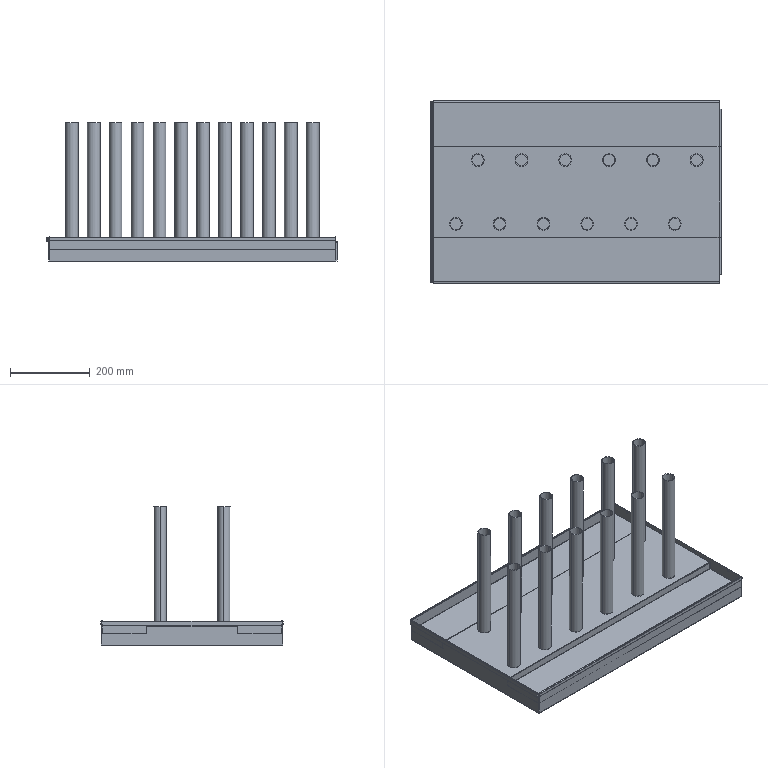Part | STEP file | RJWD-DY-0107--0001 | 14 solids | 254 faces | box 728.7 x 458 x 349.2 mm | volume 1552661 mm3 | plane 148 | cylinder 106 | commonest cylinder face diameters 29 x48 32 x24 2.4 x14 5 x8 8 x6 1.6 x2